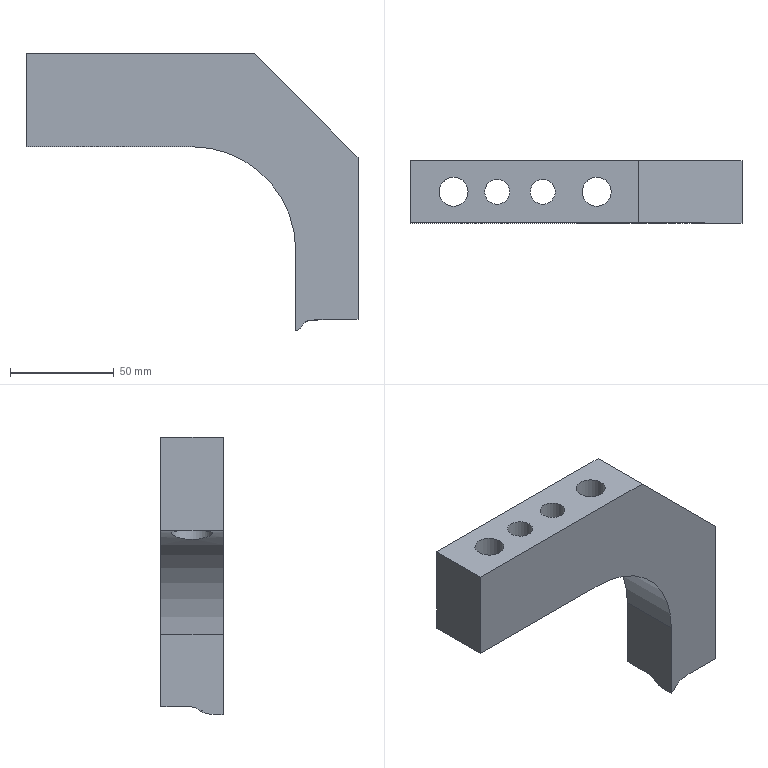Part | NX | features solid 2 | 1 solid | 24 faces | box 160 x 30 x 133.546 mm | volume 238762 mm3 | plane 10 | cylinder 7 | spline 7 | commonest cylinder face diameters 12 x2 14 x2 20 x2 100 x1